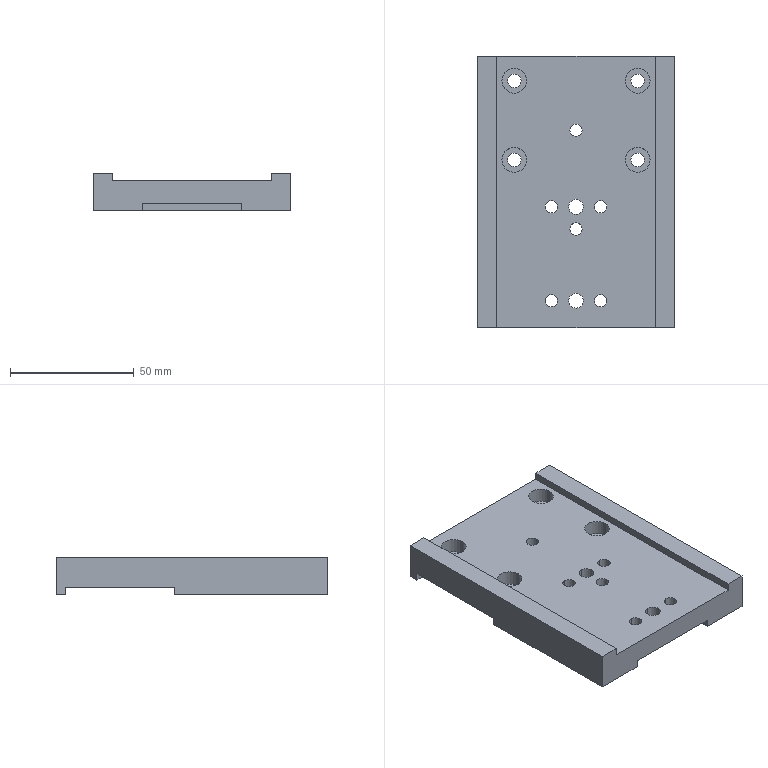Part | STEP file | X77-02301 | 1 solid | 54 faces | box 80 x 110 x 15 mm | volume 89141 mm3 | cylinder 32 | plane 22 | commonest cylinder face diameters 5 x12 5.5 x8 10 x8 6 x4